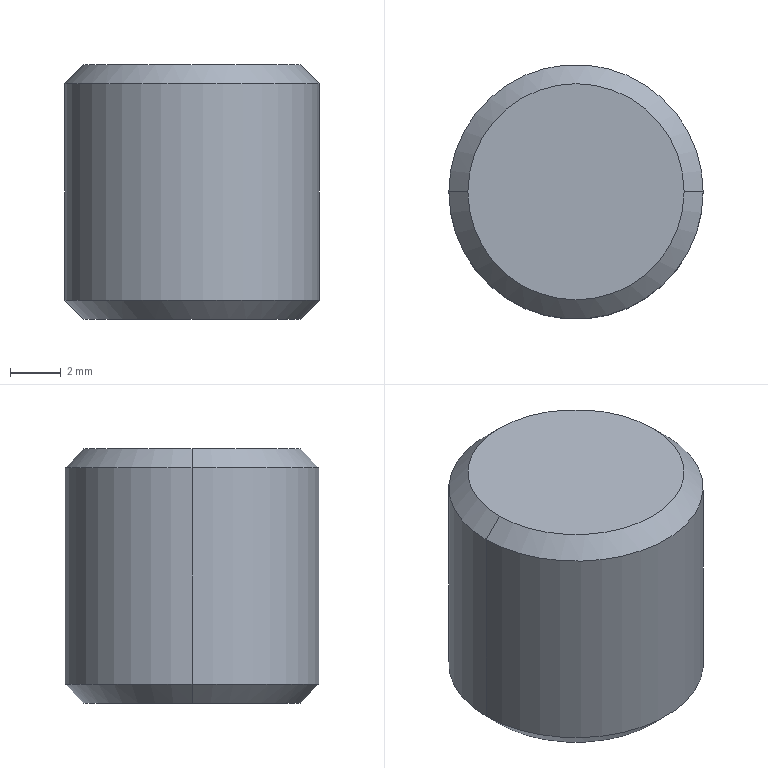Part | Creo | 1 solid | 15 faces | box 10 x 10 x 10 mm | volume 581.549 mm3 | plane 9 | cone 4 | cylinder 2 | commonest cylinder face diameters 10 x2
STEP:
#1=CARTESIAN_POINT('',(77.096,-142.631,-335.5));
#2=VERTEX_POINT('',#1);
#3=CARTESIAN_POINT('',(85.596,-142.631,-335.5));
#4=VERTEX_POINT('',#3);
#5=CARTESIAN_POINT('',(81.346,-142.631,-335.5));
#6=DIRECTION('',(0.,0.,-1.));
#7=DIRECTION('',(-1.,0.,0.));
#8=AXIS2_PLACEMENT_3D('',#5,#6,#7);
#9=CIRCLE('',#8,4.25);
#10=EDGE_CURVE('',#2,#4,#9,.T.);
#11=ORIENTED_EDGE('',*,*,#10,.F.);
#12=CARTESIAN_POINT('',(81.346,-142.631,-335.5));
#13=DIRECTION('',(0.,0.,-1.));
#14=DIRECTION('',(1.,0.,0.));
#15=AXIS2_PLACEMENT_3D('',#12,#13,#14);
#16=CIRCLE('',#15,4.25);
#17=EDGE_CURVE('',#4,#2,#16,.T.);
#18=ORIENTED_EDGE('',*,*,#17,.F.);
#19=EDGE_LOOP('',(#11,#18));
#20=FACE_OUTER_BOUND('',#19,.F.);
#21=CARTESIAN_POINT('',(78.346,-144.363,-335.5));
#22=VERTEX_POINT('',#21);
#23=CARTESIAN_POINT('',(81.346,-146.096,-335.5));
#24=VERTEX_POINT('',#23);
#25=CARTESIAN_POINT('',(78.346,-144.363,-335.5));
#26=DIRECTION('',(0.866,-0.5,0.));
#27=VECTOR('',#26,3.464);
#28=LINE('',#25,#27);
#29=EDGE_CURVE('',#22,#24,#28,.T.);
#30=ORIENTED_EDGE('',*,*,#29,.F.);
#31=CARTESIAN_POINT('',(78.346,-140.899,-335.5));
#32=VERTEX_POINT('',#31);
#33=CARTESIAN_POINT('',(78.346,-144.363,-335.5));
#34=DIRECTION('',(0.,1.,0.));
#35=VECTOR('',#34,3.464);
#36=LINE('',#33,#35);
#37=EDGE_CURVE('',#22,#32,#36,.T.);
#38=ORIENTED_EDGE('',*,*,#37,.T.);
#39=CARTESIAN_POINT('',(81.346,-139.167,-335.5));
#40=VERTEX_POINT('',#39);
#41=CARTESIAN_POINT('',(81.346,-139.167,-335.5));
#42=DIRECTION('',(-0.866,-0.5,0.));
#43=VECTOR('',#42,3.464);
#44=LINE('',#41,#43);
#45=EDGE_CURVE('',#40,#32,#44,.T.);
#46=ORIENTED_EDGE('',*,*,#45,.F.);
#47=CARTESIAN_POINT('',(84.346,-140.899,-335.5));
#48=VERTEX_POINT('',#47);
#49=CARTESIAN_POINT('',(84.346,-140.899,-335.5));
#50=DIRECTION('',(-0.866,0.5,0.));
#51=VECTOR('',#50,3.464);
#52=LINE('',#49,#51);
#53=EDGE_CURVE('',#48,#40,#52,.T.);
#54=ORIENTED_EDGE('',*,*,#53,.F.);
#55=CARTESIAN_POINT('',(84.346,-144.363,-335.5));
#56=VERTEX_POINT('',#55);
#57=CARTESIAN_POINT('',(84.346,-140.899,-335.5));
#58=DIRECTION('',(0.,-1.,0.));
#59=VECTOR('',#58,3.464);
#60=LINE('',#57,#59);
#61=EDGE_CURVE('',#48,#56,#60,.T.);
#62=ORIENTED_EDGE('',*,*,#61,.T.);
#63=CARTESIAN_POINT('',(81.346,-146.096,-335.5));
#64=DIRECTION('',(0.866,0.5,0.));
#65=VECTOR('',#64,3.464);
#66=LINE('',#63,#65);
#67=EDGE_CURVE('',#24,#56,#66,.T.);
#68=ORIENTED_EDGE('',*,*,#67,.F.);
#69=EDGE_LOOP('',(#30,#38,#46,#54,#62,#68));
#70=FACE_BOUND('',#69,.F.);
#71=CARTESIAN_POINT('',(81.346,-142.631,-335.5));
#72=DIRECTION('',(0.,0.,-1.));
#73=DIRECTION('',(-1.,0.,0.));
#74=AXIS2_PLACEMENT_3D('',#71,#72,#73);
#75=PLANE('',#74);
#76=ADVANCED_FACE('',(#20,#70),#75,.T.);
#77=ORIENTED_EDGE('',*,*,#10,.T.);
#78=CARTESIAN_POINT('',(86.346,-142.631,-334.75));
#79=VERTEX_POINT('',#78);
#80=CARTESIAN_POINT('',(85.596,-142.631,-335.5));
#81=DIRECTION('',(0.7071,0.,0.7071));
#82=VECTOR('',#81,1.061);
#83=LINE('',#80,#82);
#84=EDGE_CURVE('',#4,#79,#83,.T.);
#85=ORIENTED_EDGE('',*,*,#84,.T.);
#86=CARTESIAN_POINT('',(76.346,-142.631,-334.75));
#87=VERTEX_POINT('',#86);
#88=CARTESIAN_POINT('',(81.346,-142.631,-334.75));
#89=DIRECTION('',(0.,0.,-1.));
#90=DIRECTION('',(-1.,0.,0.));
#91=AXIS2_PLACEMENT_3D('',#88,#89,#90);
#92=CIRCLE('',#91,5.);
#93=EDGE_CURVE('',#87,#79,#92,.T.);
#94=ORIENTED_EDGE('',*,*,#93,.F.);
#95=CARTESIAN_POINT('',(77.096,-142.631,-335.5));
#96=DIRECTION('',(-0.7071,0.,0.7071));
#97=VECTOR('',#96,1.061);
#98=LINE('',#95,#97);
#99=EDGE_CURVE('',#2,#87,#98,.T.);
#100=ORIENTED_EDGE('',*,*,#99,.F.);
#101=EDGE_LOOP('',(#77,#85,#94,#100));
#102=FACE_OUTER_BOUND('',#101,.F.);
#103=CARTESIAN_POINT('',(81.346,-142.631,-335.125));
#104=DIRECTION('',(0.,0.,1.));
#105=DIRECTION('',(1.,0.,0.));
#106=AXIS2_PLACEMENT_3D('',#103,#104,#105);
#107=CONICAL_SURFACE('',#106,4.625,45.);
#108=ADVANCED_FACE('',(#102),#107,.T.);
#109=ORIENTED_EDGE('',*,*,#17,.T.);
#110=ORIENTED_EDGE('',*,*,#99,.T.);
#111=CARTESIAN_POINT('',(81.346,-142.631,-334.75));
#112=DIRECTION('',(0.,0.,-1.));
#113=DIRECTION('',(1.,0.,0.));
#114=AXIS2_PLACEMENT_3D('',#111,#112,#113);
#115=CIRCLE('',#114,5.);
#116=EDGE_CURVE('',#79,#87,#115,.T.);
#117=ORIENTED_EDGE('',*,*,#116,.F.);
#118=ORIENTED_EDGE('',*,*,#84,.F.);
#119=EDGE_LOOP('',(#109,#110,#117,#118));
#120=FACE_OUTER_BOUND('',#119,.F.);
#121=CARTESIAN_POINT('',(81.346,-142.631,-335.125));
#122=DIRECTION('',(0.,0.,1.));
#123=DIRECTION('',(1.,0.,0.));
#124=AXIS2_PLACEMENT_3D('',#121,#122,#123);
#125=CONICAL_SURFACE('',#124,4.625,45.);
#126=ADVANCED_FACE('',(#120),#125,.T.);
#127=ORIENTED_EDGE('',*,*,#116,.T.);
#128=CARTESIAN_POINT('',(76.346,-142.631,-326.25));
#129=VERTEX_POINT('',#128);
#130=CARTESIAN_POINT('',(76.346,-142.631,-326.25));
#131=DIRECTION('',(0.,0.,-1.));
#132=VECTOR('',#131,8.5);
#133=LINE('',#130,#132);
#134=EDGE_CURVE('',#129,#87,#133,.T.);
#135=ORIENTED_EDGE('',*,*,#134,.F.);
#136=CARTESIAN_POINT('',(86.346,-142.631,-326.25));
#137=VERTEX_POINT('',#136);
#138=CARTESIAN_POINT('',(81.346,-142.631,-326.25));
#139=DIRECTION('',(0.,0.,1.));
#140=DIRECTION('',(-1.,0.,0.));
#141=AXIS2_PLACEMENT_3D('',#138,#139,#140);
#142=CIRCLE('',#141,5.);
#143=EDGE_CURVE('',#129,#137,#142,.T.);
#144=ORIENTED_EDGE('',*,*,#143,.T.);
#145=CARTESIAN_POINT('',(86.346,-142.631,-326.25));
#146=DIRECTION('',(0.,0.,-1.));
#147=VECTOR('',#146,8.5);
#148=LINE('',#145,#147);
#149=EDGE_CURVE('',#137,#79,#148,.T.);
#150=ORIENTED_EDGE('',*,*,#149,.T.);
#151=EDGE_LOOP('',(#127,#135,#144,#150));
#152=FACE_OUTER_BOUND('',#151,.F.);
#153=CARTESIAN_POINT('',(81.346,-142.631,-325.5));
#154=DIRECTION('',(0.,0.,-1.));
#155=DIRECTION('',(-1.,0.,0.));
#156=AXIS2_PLACEMENT_3D('',#153,#154,#155);
#157=CYLINDRICAL_SURFACE('',#156,5.);
#158=ADVANCED_FACE('',(#152),#157,.T.);
#159=ORIENTED_EDGE('',*,*,#93,.T.);
#160=ORIENTED_EDGE('',*,*,#149,.F.);
#161=CARTESIAN_POINT('',(81.346,-142.631,-326.25));
#162=DIRECTION('',(0.,0.,1.));
#163=DIRECTION('',(1.,0.,0.));
#164=AXIS2_PLACEMENT_3D('',#161,#162,#163);
#165=CIRCLE('',#164,5.);
#166=EDGE_CURVE('',#137,#129,#165,.T.);
#167=ORIENTED_EDGE('',*,*,#166,.T.);
#168=ORIENTED_EDGE('',*,*,#134,.T.);
#169=EDGE_LOOP('',(#159,#160,#167,#168));
#170=FACE_OUTER_BOUND('',#169,.F.);
#171=CARTESIAN_POINT('',(81.346,-142.631,-325.5));
#172=DIRECTION('',(0.,0.,-1.));
#173=DIRECTION('',(-1.,0.,0.));
#174=AXIS2_PLACEMENT_3D('',#171,#172,#173);
#175=CYLINDRICAL_SURFACE('',#174,5.);
#176=ADVANCED_FACE('',(#170),#175,.T.);
#177=CARTESIAN_POINT('',(85.596,-142.631,-325.5));
#178=VERTEX_POINT('',#177);
#179=CARTESIAN_POINT('',(77.096,-142.631,-325.5));
#180=VERTEX_POINT('',#179);
#181=CARTESIAN_POINT('',(81.346,-142.631,-325.5));
#182=DIRECTION('',(0.,0.,1.));
#183=DIRECTION('',(1.,0.,0.));
#184=AXIS2_PLACEMENT_3D('',#181,#182,#183);
#185=CIRCLE('',#184,4.25);
#186=EDGE_CURVE('',#178,#180,#185,.T.);
#187=ORIENTED_EDGE('',*,*,#186,.T.);
#188=CARTESIAN_POINT('',(77.096,-142.631,-325.5));
#189=DIRECTION('',(-0.7071,0.,-0.7071));
#190=VECTOR('',#189,1.061);
#191=LINE('',#188,#190);
#192=EDGE_CURVE('',#180,#129,#191,.T.);
#193=ORIENTED_EDGE('',*,*,#192,.T.);
#194=ORIENTED_EDGE('',*,*,#166,.F.);
#195=CARTESIAN_POINT('',(85.596,-142.631,-325.5));
#196=DIRECTION('',(0.7071,0.,-0.7071));
#197=VECTOR('',#196,1.061);
#198=LINE('',#195,#197);
#199=EDGE_CURVE('',#178,#137,#198,.T.);
#200=ORIENTED_EDGE('',*,*,#199,.F.);
#201=EDGE_LOOP('',(#187,#193,#194,#200));
#202=FACE_OUTER_BOUND('',#201,.F.);
#203=CARTESIAN_POINT('',(81.346,-142.631,-325.875));
#204=DIRECTION('',(0.,0.,-1.));
#205=DIRECTION('',(-1.,0.,0.));
#206=AXIS2_PLACEMENT_3D('',#203,#204,#205);
#207=CONICAL_SURFACE('',#206,4.625,45.);
#208=ADVANCED_FACE('',(#202),#207,.T.);
#209=ORIENTED_EDGE('',*,*,#186,.F.);
#210=CARTESIAN_POINT('',(81.346,-142.631,-325.5));
#211=DIRECTION('',(0.,0.,1.));
#212=DIRECTION('',(-1.,0.,0.));
#213=AXIS2_PLACEMENT_3D('',#210,#211,#212);
#214=CIRCLE('',#213,4.25);
#215=EDGE_CURVE('',#180,#178,#214,.T.);
#216=ORIENTED_EDGE('',*,*,#215,.F.);
#217=EDGE_LOOP('',(#209,#216));
#218=FACE_OUTER_BOUND('',#217,.F.);
#219=CARTESIAN_POINT('',(81.346,-142.631,-325.5));
#220=DIRECTION('',(0.,0.,1.));
#221=DIRECTION('',(1.,0.,0.));
#222=AXIS2_PLACEMENT_3D('',#219,#220,#221);
#223=PLANE('',#222);
#224=ADVANCED_FACE('',(#218),#223,.T.);
#225=ORIENTED_EDGE('',*,*,#215,.T.);
#226=ORIENTED_EDGE('',*,*,#199,.T.);
#227=ORIENTED_EDGE('',*,*,#143,.F.);
#228=ORIENTED_EDGE('',*,*,#192,.F.);
#229=EDGE_LOOP('',(#225,#226,#227,#228));
#230=FACE_OUTER_BOUND('',#229,.F.);
#231=CARTESIAN_POINT('',(81.346,-142.631,-325.875));
#232=DIRECTION('',(0.,0.,-1.));
#233=DIRECTION('',(-1.,0.,0.));
#234=AXIS2_PLACEMENT_3D('',#231,#232,#233);
#235=CONICAL_SURFACE('',#234,4.625,45.);
#236=ADVANCED_FACE('',(#230),#235,.T.);
#237=CARTESIAN_POINT('',(81.346,-146.096,-329.5));
#238=VERTEX_POINT('',#237);
#239=CARTESIAN_POINT('',(78.346,-144.363,-329.5));
#240=VERTEX_POINT('',#239);
#241=CARTESIAN_POINT('',(81.346,-146.096,-329.5));
#242=DIRECTION('',(-0.866,0.5,0.));
#243=VECTOR('',#242,3.464);
#244=LINE('',#241,#243);
#245=EDGE_CURVE('',#238,#240,#244,.T.);
#246=ORIENTED_EDGE('',*,*,#245,.T.);
#247=CARTESIAN_POINT('',(78.346,-144.363,-329.5));
#248=DIRECTION('',(0.,0.,-1.));
#249=VECTOR('',#248,6.);
#250=LINE('',#247,#249);
#251=EDGE_CURVE('',#240,#22,#250,.T.);
#252=ORIENTED_EDGE('',*,*,#251,.T.);
#253=ORIENTED_EDGE('',*,*,#29,.T.);
#254=CARTESIAN_POINT('',(81.346,-146.096,-329.5));
#255=DIRECTION('',(0.,0.,-1.));
#256=VECTOR('',#255,6.);
#257=LINE('',#254,#256);
#258=EDGE_CURVE('',#238,#24,#257,.T.);
#259=ORIENTED_EDGE('',*,*,#258,.F.);
#260=EDGE_LOOP('',(#246,#252,#253,#259));
#261=FACE_OUTER_BOUND('',#260,.F.);
#262=CARTESIAN_POINT('',(79.846,-145.23,-332.5));
#263=DIRECTION('',(-0.5,-0.866,0.));
#264=DIRECTION('',(0.866,-0.5,0.));
#265=AXIS2_PLACEMENT_3D('',#262,#263,#264);
#266=PLANE('',#265);
#267=ADVANCED_FACE('',(#261),#266,.F.);
#268=CARTESIAN_POINT('',(78.346,-140.899,-329.5));
#269=VERTEX_POINT('',#268);
#270=CARTESIAN_POINT('',(78.346,-144.363,-329.5));
#271=DIRECTION('',(0.,1.,0.));
#272=VECTOR('',#271,3.464);
#273=LINE('',#270,#272);
#274=EDGE_CURVE('',#240,#269,#273,.T.);
#275=ORIENTED_EDGE('',*,*,#274,.F.);
#276=ORIENTED_EDGE('',*,*,#245,.F.);
#277=CARTESIAN_POINT('',(84.346,-144.363,-329.5));
#278=VERTEX_POINT('',#277);
#279=CARTESIAN_POINT('',(84.346,-144.363,-329.5));
#280=DIRECTION('',(-0.866,-0.5,0.));
#281=VECTOR('',#280,3.464);
#282=LINE('',#279,#281);
#283=EDGE_CURVE('',#278,#238,#282,.T.);
#284=ORIENTED_EDGE('',*,*,#283,.F.);
#285=CARTESIAN_POINT('',(84.346,-140.899,-329.5));
#286=VERTEX_POINT('',#285);
#287=CARTESIAN_POINT('',(84.346,-140.899,-329.5));
#288=DIRECTION('',(0.,-1.,0.));
#289=VECTOR('',#288,3.464);
#290=LINE('',#287,#289);
#291=EDGE_CURVE('',#286,#278,#290,.T.);
#292=ORIENTED_EDGE('',*,*,#291,.F.);
#293=CARTESIAN_POINT('',(81.346,-139.167,-329.5));
#294=VERTEX_POINT('',#293);
#295=CARTESIAN_POINT('',(81.346,-139.167,-329.5));
#296=DIRECTION('',(0.866,-0.5,0.));
#297=VECTOR('',#296,3.464);
#298=LINE('',#295,#297);
#299=EDGE_CURVE('',#294,#286,#298,.T.);
#300=ORIENTED_EDGE('',*,*,#299,.F.);
#301=CARTESIAN_POINT('',(78.346,-140.899,-329.5));
#302=DIRECTION('',(0.866,0.5,0.));
#303=VECTOR('',#302,3.464);
#304=LINE('',#301,#303);
#305=EDGE_CURVE('',#269,#294,#304,.T.);
#306=ORIENTED_EDGE('',*,*,#305,.F.);
#307=EDGE_LOOP('',(#275,#276,#284,#292,#300,#306));
#308=FACE_OUTER_BOUND('',#307,.F.);
#309=CARTESIAN_POINT('',(81.346,-142.631,-329.5));
#310=DIRECTION('',(0.,0.,1.));
#311=DIRECTION('',(1.,0.,0.));
#312=AXIS2_PLACEMENT_3D('',#309,#310,#311);
#313=PLANE('',#312);
#314=ADVANCED_FACE('',(#308),#313,.F.);
#315=ORIENTED_EDGE('',*,*,#274,.T.);
#316=CARTESIAN_POINT('',(78.346,-140.899,-329.5));
#317=DIRECTION('',(0.,0.,-1.));
#318=VECTOR('',#317,6.);
#319=LINE('',#316,#318);
#320=EDGE_CURVE('',#269,#32,#319,.T.);
#321=ORIENTED_EDGE('',*,*,#320,.T.);
#322=ORIENTED_EDGE('',*,*,#37,.F.);
#323=ORIENTED_EDGE('',*,*,#251,.F.);
#324=EDGE_LOOP('',(#315,#321,#322,#323));
#325=FACE_OUTER_BOUND('',#324,.F.);
#326=CARTESIAN_POINT('',(78.346,-142.631,-332.5));
#327=DIRECTION('',(-1.,0.,0.));
#328=DIRECTION('',(0.,0.,1.));
#329=AXIS2_PLACEMENT_3D('',#326,#327,#328);
#330=PLANE('',#329);
#331=ADVANCED_FACE('',(#325),#330,.F.);
#332=ORIENTED_EDGE('',*,*,#305,.T.);
#333=CARTESIAN_POINT('',(81.346,-139.167,-329.5));
#334=DIRECTION('',(0.,0.,-1.));
#335=VECTOR('',#334,6.);
#336=LINE('',#333,#335);
#337=EDGE_CURVE('',#294,#40,#336,.T.);
#338=ORIENTED_EDGE('',*,*,#337,.T.);
#339=ORIENTED_EDGE('',*,*,#45,.T.);
#340=ORIENTED_EDGE('',*,*,#320,.F.);
#341=EDGE_LOOP('',(#332,#338,#339,#340));
#342=FACE_OUTER_BOUND('',#341,.F.);
#343=CARTESIAN_POINT('',(79.846,-140.033,-332.5));
#344=DIRECTION('',(-0.5,0.866,0.));
#345=DIRECTION('',(-0.866,-0.5,0.));
#346=AXIS2_PLACEMENT_3D('',#343,#344,#345);
#347=PLANE('',#346);
#348=ADVANCED_FACE('',(#342),#347,.F.);
#349=ORIENTED_EDGE('',*,*,#299,.T.);
#350=CARTESIAN_POINT('',(84.346,-140.899,-329.5));
#351=DIRECTION('',(0.,0.,-1.));
#352=VECTOR('',#351,6.);
#353=LINE('',#350,#352);
#354=EDGE_CURVE('',#286,#48,#353,.T.);
#355=ORIENTED_EDGE('',*,*,#354,.T.);
#356=ORIENTED_EDGE('',*,*,#53,.T.);
#357=ORIENTED_EDGE('',*,*,#337,.F.);
#358=EDGE_LOOP('',(#349,#355,#356,#357));
#359=FACE_OUTER_BOUND('',#358,.F.);
#360=CARTESIAN_POINT('',(82.846,-140.033,-332.5));
#361=DIRECTION('',(0.5,0.866,0.));
#362=DIRECTION('',(-0.866,0.5,0.));
#363=AXIS2_PLACEMENT_3D('',#360,#361,#362);
#364=PLANE('',#363);
#365=ADVANCED_FACE('',(#359),#364,.F.);
#366=ORIENTED_EDGE('',*,*,#291,.T.);
#367=CARTESIAN_POINT('',(84.346,-144.363,-329.5));
#368=DIRECTION('',(0.,0.,-1.));
#369=VECTOR('',#368,6.);
#370=LINE('',#367,#369);
#371=EDGE_CURVE('',#278,#56,#370,.T.);
#372=ORIENTED_EDGE('',*,*,#371,.T.);
#373=ORIENTED_EDGE('',*,*,#61,.F.);
#374=ORIENTED_EDGE('',*,*,#354,.F.);
#375=EDGE_LOOP('',(#366,#372,#373,#374));
#376=FACE_OUTER_BOUND('',#375,.F.);
#377=CARTESIAN_POINT('',(84.346,-142.631,-332.5));
#378=DIRECTION('',(1.,0.,0.));
#379=DIRECTION('',(0.,0.,-1.));
#380=AXIS2_PLACEMENT_3D('',#377,#378,#379);
#381=PLANE('',#380);
#382=ADVANCED_FACE('',(#376),#381,.F.);
#383=ORIENTED_EDGE('',*,*,#283,.T.);
#384=ORIENTED_EDGE('',*,*,#258,.T.);
#385=ORIENTED_EDGE('',*,*,#67,.T.);
#386=ORIENTED_EDGE('',*,*,#371,.F.);
#387=EDGE_LOOP('',(#383,#384,#385,#386));
#388=FACE_OUTER_BOUND('',#387,.F.);
#389=CARTESIAN_POINT('',(82.846,-145.23,-332.5));
#390=DIRECTION('',(0.5,-0.866,0.));
#391=DIRECTION('',(0.866,0.5,0.));
#392=AXIS2_PLACEMENT_3D('',#389,#390,#391);
#393=PLANE('',#392);
#394=ADVANCED_FACE('',(#388),#393,.F.);
#395=CLOSED_SHELL('',(#76,#108,#126,#158,#176,#208,#224,#236,#267,#314,#331,#348,#365,#382,#394));
#396=MANIFOLD_SOLID_BREP('',#395);
#397=(LENGTH_UNIT()NAMED_UNIT(*)SI_UNIT(.MILLI.,.METRE.));
#398=UNCERTAINTY_MEASURE_WITH_UNIT(LENGTH_MEASURE(0.001732),#397,'','');
#399=(NAMED_UNIT(*)PLANE_ANGLE_UNIT()SI_UNIT($,.RADIAN.));
#400=PLANE_ANGLE_MEASURE_WITH_UNIT(PLANE_ANGLE_MEASURE(0.01745),#399);
#401=(CONVERSION_BASED_UNIT('DEGREE',#400)NAMED_UNIT(*)PLANE_ANGLE_UNIT());
#402=(NAMED_UNIT(*)SI_UNIT($,.STERADIAN.)SOLID_ANGLE_UNIT());
#403=(GEOMETRIC_REPRESENTATION_CONTEXT(3)GLOBAL_UNCERTAINTY_ASSIGNED_CONTEXT((#398))GLOBAL_UNIT_ASSIGNED_CONTEXT((#397,#401,#402))REPRESENTATION_CONTEXT('',''));
#404=ADVANCED_BREP_SHAPE_REPRESENTATION('',(#396),#403);